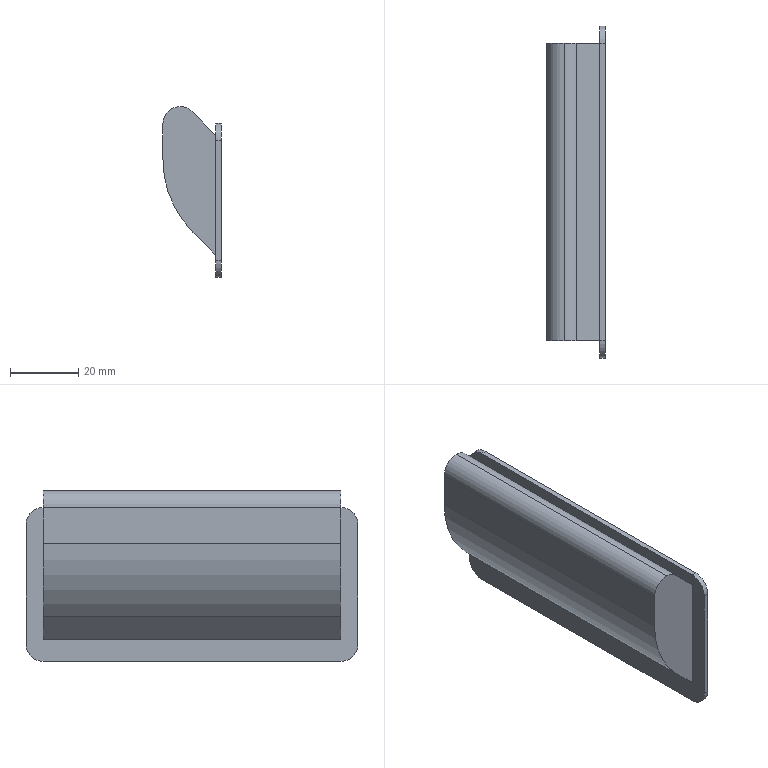Part | SolidWorks | features BaseBody 1 | 1 solid | 23 faces | box 17 x 97 x 49.929 mm | volume 24754 mm3 | plane 14 | cylinder 9 | commonest cylinder face diameters 10 x6 30 x2 60 x1
STEP:
#1=CARTESIAN_POINT('',(5.,-43.5,10.429));
#2=VERTEX_POINT('',#1);
#3=CARTESIAN_POINT('',(0.,-43.5,5.429));
#4=VERTEX_POINT('',#3);
#5=CARTESIAN_POINT('',(5.,-43.5,5.429));
#6=DIRECTION('',(0.,-1.,0.));
#7=DIRECTION('',(0.,0.,1.));
#8=AXIS2_PLACEMENT_3D('',#5,#6,#7);
#9=CIRCLE('',#8,5.);
#10=EDGE_CURVE('',#2,#4,#9,.T.);
#11=ORIENTED_EDGE('',*,*,#10,.F.);
#12=CARTESIAN_POINT('',(5.,43.5,10.429));
#13=VERTEX_POINT('',#12);
#14=CARTESIAN_POINT('',(5.,-43.5,10.429));
#15=DIRECTION('',(0.,1.,0.));
#16=VECTOR('',#15,1000.);
#17=LINE('',#14,#16);
#18=EDGE_CURVE('',#2,#13,#17,.T.);
#19=ORIENTED_EDGE('',*,*,#18,.T.);
#20=CARTESIAN_POINT('',(0.,43.5,5.429));
#21=VERTEX_POINT('',#20);
#22=CARTESIAN_POINT('',(5.,43.5,5.429));
#23=DIRECTION('',(0.,-1.,0.));
#24=DIRECTION('',(0.,0.,1.));
#25=AXIS2_PLACEMENT_3D('',#22,#23,#24);
#26=CIRCLE('',#25,5.);
#27=EDGE_CURVE('',#13,#21,#26,.T.);
#28=ORIENTED_EDGE('',*,*,#27,.T.);
#29=CARTESIAN_POINT('',(0.,-43.5,5.429));
#30=DIRECTION('',(0.,1.,0.));
#31=VECTOR('',#30,1000.);
#32=LINE('',#29,#31);
#33=EDGE_CURVE('',#4,#21,#32,.T.);
#34=ORIENTED_EDGE('',*,*,#33,.F.);
#35=EDGE_LOOP('',(#11,#19,#28,#34));
#36=FACE_OUTER_BOUND('',#35,.T.);
#37=CARTESIAN_POINT('',(5.,-43.5,5.429));
#38=DIRECTION('',(0.,1.,0.));
#39=DIRECTION('',(0.,0.,1.));
#40=AXIS2_PLACEMENT_3D('',#37,#38,#39);
#41=CYLINDRICAL_SURFACE('',#40,5.);
#42=ADVANCED_FACE('',(#36),#41,.T.);
#43=CARTESIAN_POINT('',(8.787,-43.5,-26.287));
#44=VERTEX_POINT('',#43);
#45=CARTESIAN_POINT('',(0.,-43.5,-5.074));
#46=VERTEX_POINT('',#45);
#47=CARTESIAN_POINT('',(30.,-43.5,-5.074));
#48=DIRECTION('',(0.,1.,0.));
#49=DIRECTION('',(0.,0.,1.));
#50=AXIS2_PLACEMENT_3D('',#47,#48,#49);
#51=CIRCLE('',#50,30.);
#52=EDGE_CURVE('',#44,#46,#51,.T.);
#53=ORIENTED_EDGE('',*,*,#52,.T.);
#54=CARTESIAN_POINT('',(0.,43.5,-5.074));
#55=VERTEX_POINT('',#54);
#56=CARTESIAN_POINT('',(0.,-43.5,-5.074));
#57=DIRECTION('',(0.,1.,0.));
#58=VECTOR('',#57,1000.);
#59=LINE('',#56,#58);
#60=EDGE_CURVE('',#46,#55,#59,.T.);
#61=ORIENTED_EDGE('',*,*,#60,.T.);
#62=CARTESIAN_POINT('',(8.787,43.5,-26.287));
#63=VERTEX_POINT('',#62);
#64=CARTESIAN_POINT('',(30.,43.5,-5.074));
#65=DIRECTION('',(0.,-1.,0.));
#66=DIRECTION('',(0.,0.,1.));
#67=AXIS2_PLACEMENT_3D('',#64,#65,#66);
#68=CIRCLE('',#67,30.);
#69=EDGE_CURVE('',#55,#63,#68,.T.);
#70=ORIENTED_EDGE('',*,*,#69,.T.);
#71=CARTESIAN_POINT('',(8.787,-43.5,-26.287));
#72=DIRECTION('',(0.,-1.,0.));
#73=VECTOR('',#72,1000.);
#74=LINE('',#71,#73);
#75=EDGE_CURVE('',#63,#44,#74,.T.);
#76=ORIENTED_EDGE('',*,*,#75,.T.);
#77=EDGE_LOOP('',(#53,#61,#70,#76));
#78=FACE_OUTER_BOUND('',#77,.T.);
#79=CARTESIAN_POINT('',(30.,-43.5,-5.074));
#80=DIRECTION('',(0.,1.,0.));
#81=DIRECTION('',(0.,0.,1.));
#82=AXIS2_PLACEMENT_3D('',#79,#80,#81);
#83=CYLINDRICAL_SURFACE('',#82,30.);
#84=ADVANCED_FACE('',(#78),#83,.T.);
#85=CARTESIAN_POINT('',(0.,43.5,-17.5));
#86=DIRECTION('',(0.,0.,-1.));
#87=VECTOR('',#86,1000.);
#88=LINE('',#85,#87);
#89=EDGE_CURVE('',#21,#55,#88,.T.);
#90=ORIENTED_EDGE('',*,*,#89,.T.);
#91=ORIENTED_EDGE('',*,*,#60,.F.);
#92=CARTESIAN_POINT('',(0.,-43.5,-17.5));
#93=DIRECTION('',(0.,0.,1.));
#94=VECTOR('',#93,1000.);
#95=LINE('',#92,#94);
#96=EDGE_CURVE('',#46,#4,#95,.T.);
#97=ORIENTED_EDGE('',*,*,#96,.T.);
#98=ORIENTED_EDGE('',*,*,#33,.T.);
#99=EDGE_LOOP('',(#90,#91,#97,#98));
#100=FACE_OUTER_BOUND('',#99,.T.);
#101=CARTESIAN_POINT('',(0.,-43.5,-17.5));
#102=DIRECTION('',(-1.,0.,0.));
#103=DIRECTION('',(0.,0.,1.));
#104=AXIS2_PLACEMENT_3D('',#101,#102,#103);
#105=PLANE('',#104);
#106=ADVANCED_FACE('',(#100),#105,.T.);
#107=CARTESIAN_POINT('',(8.536,-43.5,8.964));
#108=VERTEX_POINT('',#107);
#109=CARTESIAN_POINT('',(5.,-43.5,5.429));
#110=DIRECTION('',(0.,-1.,0.));
#111=DIRECTION('',(0.,0.,1.));
#112=AXIS2_PLACEMENT_3D('',#109,#110,#111);
#113=CIRCLE('',#112,5.);
#114=EDGE_CURVE('',#108,#2,#113,.T.);
#115=ORIENTED_EDGE('',*,*,#114,.T.);
#116=ORIENTED_EDGE('',*,*,#10,.T.);
#117=ORIENTED_EDGE('',*,*,#96,.F.);
#118=ORIENTED_EDGE('',*,*,#52,.F.);
#119=CARTESIAN_POINT('',(15.5,-43.5,-33.));
#120=VERTEX_POINT('',#119);
#121=CARTESIAN_POINT('',(8.787,-43.5,-26.287));
#122=DIRECTION('',(0.7071,0.,-0.7071));
#123=VECTOR('',#122,1000.);
#124=LINE('',#121,#123);
#125=EDGE_CURVE('',#44,#120,#124,.T.);
#126=ORIENTED_EDGE('',*,*,#125,.T.);
#127=CARTESIAN_POINT('',(15.5,-43.5,2.));
#128=VERTEX_POINT('',#127);
#129=CARTESIAN_POINT('',(15.5,-43.5,0.5));
#130=DIRECTION('',(0.,0.,1.));
#131=VECTOR('',#130,1000.);
#132=LINE('',#129,#131);
#133=EDGE_CURVE('',#120,#128,#132,.T.);
#134=ORIENTED_EDGE('',*,*,#133,.T.);
#135=CARTESIAN_POINT('',(15.5,-43.5,2.));
#136=DIRECTION('',(-0.7071,0.,0.7071));
#137=VECTOR('',#136,1000.);
#138=LINE('',#135,#137);
#139=EDGE_CURVE('',#128,#108,#138,.T.);
#140=ORIENTED_EDGE('',*,*,#139,.T.);
#141=EDGE_LOOP('',(#115,#116,#117,#118,#126,#134,#140));
#142=FACE_OUTER_BOUND('',#141,.T.);
#143=CARTESIAN_POINT('',(17.,-43.5,0.5));
#144=DIRECTION('',(0.,-1.,0.));
#145=DIRECTION('',(0.,0.,-1.));
#146=AXIS2_PLACEMENT_3D('',#143,#144,#145);
#147=PLANE('',#146);
#148=ADVANCED_FACE('',(#142),#147,.T.);
#149=CARTESIAN_POINT('',(15.5,43.5,-33.));
#150=VERTEX_POINT('',#149);
#151=CARTESIAN_POINT('',(15.5,-43.5,-33.));
#152=DIRECTION('',(0.,-1.,0.));
#153=VECTOR('',#152,1000.);
#154=LINE('',#151,#153);
#155=EDGE_CURVE('',#150,#120,#154,.T.);
#156=ORIENTED_EDGE('',*,*,#155,.T.);
#157=ORIENTED_EDGE('',*,*,#125,.F.);
#158=ORIENTED_EDGE('',*,*,#75,.F.);
#159=CARTESIAN_POINT('',(17.,43.5,-34.5));
#160=DIRECTION('',(0.7071,0.,-0.7071));
#161=VECTOR('',#160,1000.);
#162=LINE('',#159,#161);
#163=EDGE_CURVE('',#63,#150,#162,.T.);
#164=ORIENTED_EDGE('',*,*,#163,.T.);
#165=EDGE_LOOP('',(#156,#157,#158,#164));
#166=FACE_OUTER_BOUND('',#165,.T.);
#167=CARTESIAN_POINT('',(17.,-43.5,-34.5));
#168=DIRECTION('',(-0.7071,0.,-0.7071));
#169=DIRECTION('',(-0.7071,0.,0.7071));
#170=AXIS2_PLACEMENT_3D('',#167,#168,#169);
#171=PLANE('',#170);
#172=ADVANCED_FACE('',(#166),#171,.T.);
#173=ORIENTED_EDGE('',*,*,#163,.F.);
#174=ORIENTED_EDGE('',*,*,#69,.F.);
#175=ORIENTED_EDGE('',*,*,#89,.F.);
#176=ORIENTED_EDGE('',*,*,#27,.F.);
#177=CARTESIAN_POINT('',(8.536,43.5,8.964));
#178=VERTEX_POINT('',#177);
#179=CARTESIAN_POINT('',(5.,43.5,5.429));
#180=DIRECTION('',(0.,-1.,0.));
#181=DIRECTION('',(0.,0.,1.));
#182=AXIS2_PLACEMENT_3D('',#179,#180,#181);
#183=CIRCLE('',#182,5.);
#184=EDGE_CURVE('',#178,#13,#183,.T.);
#185=ORIENTED_EDGE('',*,*,#184,.F.);
#186=CARTESIAN_POINT('',(15.5,43.5,2.));
#187=VERTEX_POINT('',#186);
#188=CARTESIAN_POINT('',(15.5,43.5,2.));
#189=DIRECTION('',(-0.7071,0.,0.7071));
#190=VECTOR('',#189,1000.);
#191=LINE('',#188,#190);
#192=EDGE_CURVE('',#187,#178,#191,.T.);
#193=ORIENTED_EDGE('',*,*,#192,.F.);
#194=CARTESIAN_POINT('',(15.5,43.5,0.5));
#195=DIRECTION('',(0.,0.,1.));
#196=VECTOR('',#195,1000.);
#197=LINE('',#194,#196);
#198=EDGE_CURVE('',#150,#187,#197,.T.);
#199=ORIENTED_EDGE('',*,*,#198,.F.);
#200=EDGE_LOOP('',(#173,#174,#175,#176,#185,#193,#199));
#201=FACE_OUTER_BOUND('',#200,.T.);
#202=CARTESIAN_POINT('',(17.,43.5,0.5));
#203=DIRECTION('',(0.,-1.,0.));
#204=DIRECTION('',(0.,0.,-1.));
#205=AXIS2_PLACEMENT_3D('',#202,#203,#204);
#206=PLANE('',#205);
#207=ADVANCED_FACE('',(#201),#206,.F.);
#208=ORIENTED_EDGE('',*,*,#18,.F.);
#209=ORIENTED_EDGE('',*,*,#114,.F.);
#210=CARTESIAN_POINT('',(8.536,-43.5,8.964));
#211=DIRECTION('',(0.,1.,0.));
#212=VECTOR('',#211,1000.);
#213=LINE('',#210,#212);
#214=EDGE_CURVE('',#108,#178,#213,.T.);
#215=ORIENTED_EDGE('',*,*,#214,.T.);
#216=ORIENTED_EDGE('',*,*,#184,.T.);
#217=EDGE_LOOP('',(#208,#209,#215,#216));
#218=FACE_OUTER_BOUND('',#217,.T.);
#219=CARTESIAN_POINT('',(5.,-43.5,5.429));
#220=DIRECTION('',(0.,1.,0.));
#221=DIRECTION('',(0.,0.,1.));
#222=AXIS2_PLACEMENT_3D('',#219,#220,#221);
#223=CYLINDRICAL_SURFACE('',#222,5.);
#224=ADVANCED_FACE('',(#218),#223,.T.);
#225=CARTESIAN_POINT('',(15.5,-43.5,2.));
#226=DIRECTION('',(0.,1.,0.));
#227=VECTOR('',#226,1000.);
#228=LINE('',#225,#227);
#229=EDGE_CURVE('',#128,#187,#228,.T.);
#230=ORIENTED_EDGE('',*,*,#229,.T.);
#231=ORIENTED_EDGE('',*,*,#192,.T.);
#232=ORIENTED_EDGE('',*,*,#214,.F.);
#233=ORIENTED_EDGE('',*,*,#139,.F.);
#234=EDGE_LOOP('',(#230,#231,#232,#233));
#235=FACE_OUTER_BOUND('',#234,.T.);
#236=CARTESIAN_POINT('',(0.,-43.5,17.5));
#237=DIRECTION('',(0.7071,0.,0.7071));
#238=DIRECTION('',(0.7071,0.,-0.7071));
#239=AXIS2_PLACEMENT_3D('',#236,#237,#238);
#240=PLANE('',#239);
#241=ADVANCED_FACE('',(#235),#240,.T.);
#242=CARTESIAN_POINT('',(15.5,-43.5,5.5));
#243=VERTEX_POINT('',#242);
#244=CARTESIAN_POINT('',(15.5,43.5,5.5));
#245=VERTEX_POINT('',#244);
#246=CARTESIAN_POINT('',(15.5,48.5,5.5));
#247=DIRECTION('',(0.,1.,0.));
#248=VECTOR('',#247,1000.);
#249=LINE('',#246,#248);
#250=EDGE_CURVE('',#243,#245,#249,.T.);
#251=ORIENTED_EDGE('',*,*,#250,.T.);
#252=CARTESIAN_POINT('',(15.5,48.5,0.5));
#253=VERTEX_POINT('',#252);
#254=CARTESIAN_POINT('',(15.5,43.5,0.5));
#255=DIRECTION('',(-1.,0.,0.));
#256=DIRECTION('',(0.,0.,-1.));
#257=AXIS2_PLACEMENT_3D('',#254,#255,#256);
#258=CIRCLE('',#257,5.);
#259=EDGE_CURVE('',#245,#253,#258,.T.);
#260=ORIENTED_EDGE('',*,*,#259,.T.);
#261=CARTESIAN_POINT('',(15.5,48.5,-34.5));
#262=VERTEX_POINT('',#261);
#263=CARTESIAN_POINT('',(15.5,48.5,5.5));
#264=DIRECTION('',(0.,0.,-1.));
#265=VECTOR('',#264,1000.);
#266=LINE('',#263,#265);
#267=EDGE_CURVE('',#253,#262,#266,.T.);
#268=ORIENTED_EDGE('',*,*,#267,.T.);
#269=CARTESIAN_POINT('',(15.5,43.5,-39.5));
#270=VERTEX_POINT('',#269);
#271=CARTESIAN_POINT('',(15.5,43.5,-34.5));
#272=DIRECTION('',(-1.,0.,0.));
#273=DIRECTION('',(0.,0.,-1.));
#274=AXIS2_PLACEMENT_3D('',#271,#272,#273);
#275=CIRCLE('',#274,5.);
#276=EDGE_CURVE('',#262,#270,#275,.T.);
#277=ORIENTED_EDGE('',*,*,#276,.T.);
#278=CARTESIAN_POINT('',(15.5,-43.5,-39.5));
#279=VERTEX_POINT('',#278);
#280=CARTESIAN_POINT('',(15.5,48.5,-39.5));
#281=DIRECTION('',(0.,-1.,0.));
#282=VECTOR('',#281,1000.);
#283=LINE('',#280,#282);
#284=EDGE_CURVE('',#270,#279,#283,.T.);
#285=ORIENTED_EDGE('',*,*,#284,.T.);
#286=CARTESIAN_POINT('',(15.5,-48.5,-34.5));
#287=VERTEX_POINT('',#286);
#288=CARTESIAN_POINT('',(15.5,-43.5,-34.5));
#289=DIRECTION('',(-1.,0.,0.));
#290=DIRECTION('',(0.,0.,-1.));
#291=AXIS2_PLACEMENT_3D('',#288,#289,#290);
#292=CIRCLE('',#291,5.);
#293=EDGE_CURVE('',#279,#287,#292,.T.);
#294=ORIENTED_EDGE('',*,*,#293,.T.);
#295=CARTESIAN_POINT('',(15.5,-48.5,0.5));
#296=VERTEX_POINT('',#295);
#297=CARTESIAN_POINT('',(15.5,-48.5,5.5));
#298=DIRECTION('',(0.,0.,1.));
#299=VECTOR('',#298,1000.);
#300=LINE('',#297,#299);
#301=EDGE_CURVE('',#287,#296,#300,.T.);
#302=ORIENTED_EDGE('',*,*,#301,.T.);
#303=CARTESIAN_POINT('',(15.5,-43.5,0.5));
#304=DIRECTION('',(-1.,0.,0.));
#305=DIRECTION('',(0.,0.,-1.));
#306=AXIS2_PLACEMENT_3D('',#303,#304,#305);
#307=CIRCLE('',#306,5.);
#308=EDGE_CURVE('',#296,#243,#307,.T.);
#309=ORIENTED_EDGE('',*,*,#308,.T.);
#310=EDGE_LOOP('',(#251,#260,#268,#277,#285,#294,#302,#309));
#311=FACE_OUTER_BOUND('',#310,.T.);
#312=ORIENTED_EDGE('',*,*,#229,.F.);
#313=ORIENTED_EDGE('',*,*,#133,.F.);
#314=ORIENTED_EDGE('',*,*,#155,.F.);
#315=ORIENTED_EDGE('',*,*,#198,.T.);
#316=EDGE_LOOP('',(#312,#313,#314,#315));
#317=FACE_BOUND('',#316,.T.);
#318=CARTESIAN_POINT('',(15.5,48.5,5.5));
#319=DIRECTION('',(-1.,0.,0.));
#320=DIRECTION('',(0.,0.,1.));
#321=AXIS2_PLACEMENT_3D('',#318,#319,#320);
#322=PLANE('',#321);
#323=ADVANCED_FACE('',(#311,#317),#322,.T.);
#324=ORIENTED_EDGE('',*,*,#259,.F.);
#325=CARTESIAN_POINT('',(17.,43.5,5.5));
#326=VERTEX_POINT('',#325);
#327=CARTESIAN_POINT('',(15.5,43.5,5.5));
#328=DIRECTION('',(1.,0.,0.));
#329=VECTOR('',#328,1000.);
#330=LINE('',#327,#329);
#331=EDGE_CURVE('',#245,#326,#330,.T.);
#332=ORIENTED_EDGE('',*,*,#331,.T.);
#333=CARTESIAN_POINT('',(17.,48.5,0.5));
#334=VERTEX_POINT('',#333);
#335=CARTESIAN_POINT('',(17.,43.5,0.5));
#336=DIRECTION('',(-1.,0.,0.));
#337=DIRECTION('',(0.,0.,-1.));
#338=AXIS2_PLACEMENT_3D('',#335,#336,#337);
#339=CIRCLE('',#338,5.);
#340=EDGE_CURVE('',#326,#334,#339,.T.);
#341=ORIENTED_EDGE('',*,*,#340,.T.);
#342=CARTESIAN_POINT('',(15.5,48.5,0.5));
#343=DIRECTION('',(-1.,0.,0.));
#344=VECTOR('',#343,1000.);
#345=LINE('',#342,#344);
#346=EDGE_CURVE('',#334,#253,#345,.T.);
#347=ORIENTED_EDGE('',*,*,#346,.T.);
#348=EDGE_LOOP('',(#324,#332,#341,#347));
#349=FACE_OUTER_BOUND('',#348,.T.);
#350=CARTESIAN_POINT('',(15.5,43.5,0.5));
#351=DIRECTION('',(1.,0.,0.));
#352=DIRECTION('',(0.,0.,-1.));
#353=AXIS2_PLACEMENT_3D('',#350,#351,#352);
#354=CYLINDRICAL_SURFACE('',#353,5.);
#355=ADVANCED_FACE('',(#349),#354,.T.);
#356=ORIENTED_EDGE('',*,*,#250,.F.);
#357=CARTESIAN_POINT('',(17.,-43.5,5.5));
#358=VERTEX_POINT('',#357);
#359=CARTESIAN_POINT('',(15.5,-43.5,5.5));
#360=DIRECTION('',(-1.,0.,0.));
#361=VECTOR('',#360,1000.);
#362=LINE('',#359,#361);
#363=EDGE_CURVE('',#358,#243,#362,.T.);
#364=ORIENTED_EDGE('',*,*,#363,.F.);
#365=CARTESIAN_POINT('',(17.,-48.5,5.5));
#366=DIRECTION('',(0.,-1.,0.));
#367=VECTOR('',#366,1000.);
#368=LINE('',#365,#367);
#369=EDGE_CURVE('',#326,#358,#368,.T.);
#370=ORIENTED_EDGE('',*,*,#369,.F.);
#371=ORIENTED_EDGE('',*,*,#331,.F.);
#372=EDGE_LOOP('',(#356,#364,#370,#371));
#373=FACE_OUTER_BOUND('',#372,.T.);
#374=CARTESIAN_POINT('',(15.5,-48.5,5.5));
#375=DIRECTION('',(0.,0.,-1.));
#376=DIRECTION('',(-1.,0.,0.));
#377=AXIS2_PLACEMENT_3D('',#374,#375,#376);
#378=PLANE('',#377);
#379=ADVANCED_FACE('',(#373),#378,.F.);
#380=ORIENTED_EDGE('',*,*,#308,.F.);
#381=CARTESIAN_POINT('',(17.,-48.5,0.5));
#382=VERTEX_POINT('',#381);
#383=CARTESIAN_POINT('',(15.5,-48.5,0.5));
#384=DIRECTION('',(1.,0.,0.));
#385=VECTOR('',#384,1000.);
#386=LINE('',#383,#385);
#387=EDGE_CURVE('',#296,#382,#386,.T.);
#388=ORIENTED_EDGE('',*,*,#387,.T.);
#389=CARTESIAN_POINT('',(17.,-43.5,0.5));
#390=DIRECTION('',(-1.,0.,0.));
#391=DIRECTION('',(0.,0.,-1.));
#392=AXIS2_PLACEMENT_3D('',#389,#390,#391);
#393=CIRCLE('',#392,5.);
#394=EDGE_CURVE('',#382,#358,#393,.T.);
#395=ORIENTED_EDGE('',*,*,#394,.T.);
#396=ORIENTED_EDGE('',*,*,#363,.T.);
#397=EDGE_LOOP('',(#380,#388,#395,#396));
#398=FACE_OUTER_BOUND('',#397,.T.);
#399=CARTESIAN_POINT('',(15.5,-43.5,0.5));
#400=DIRECTION('',(1.,0.,0.));
#401=DIRECTION('',(0.,0.,-1.));
#402=AXIS2_PLACEMENT_3D('',#399,#400,#401);
#403=CYLINDRICAL_SURFACE('',#402,5.);
#404=ADVANCED_FACE('',(#398),#403,.T.);
#405=CARTESIAN_POINT('',(17.,-48.5,-34.5));
#406=VERTEX_POINT('',#405);
#407=CARTESIAN_POINT('',(17.,-48.5,-39.5));
#408=DIRECTION('',(0.,0.,-1.));
#409=VECTOR('',#408,1000.);
#410=LINE('',#407,#409);
#411=EDGE_CURVE('',#382,#406,#410,.T.);
#412=ORIENTED_EDGE('',*,*,#411,.F.);
#413=ORIENTED_EDGE('',*,*,#387,.F.);
#414=ORIENTED_EDGE('',*,*,#301,.F.);
#415=CARTESIAN_POINT('',(15.5,-48.5,-34.5));
#416=DIRECTION('',(-1.,0.,0.));
#417=VECTOR('',#416,1000.);
#418=LINE('',#415,#417);
#419=EDGE_CURVE('',#406,#287,#418,.T.);
#420=ORIENTED_EDGE('',*,*,#419,.F.);
#421=EDGE_LOOP('',(#412,#413,#414,#420));
#422=FACE_OUTER_BOUND('',#421,.T.);
#423=CARTESIAN_POINT('',(15.5,-48.5,-39.5));
#424=DIRECTION('',(0.,1.,0.));
#425=DIRECTION('',(0.,0.,1.));
#426=AXIS2_PLACEMENT_3D('',#423,#424,#425);
#427=PLANE('',#426);
#428=ADVANCED_FACE('',(#422),#427,.F.);
#429=ORIENTED_EDGE('',*,*,#293,.F.);
#430=CARTESIAN_POINT('',(17.,-43.5,-39.5));
#431=VERTEX_POINT('',#430);
#432=CARTESIAN_POINT('',(15.5,-43.5,-39.5));
#433=DIRECTION('',(1.,0.,0.));
#434=VECTOR('',#433,1000.);
#435=LINE('',#432,#434);
#436=EDGE_CURVE('',#279,#431,#435,.T.);
#437=ORIENTED_EDGE('',*,*,#436,.T.);
#438=CARTESIAN_POINT('',(17.,-43.5,-34.5));
#439=DIRECTION('',(-1.,0.,0.));
#440=DIRECTION('',(0.,0.,-1.));
#441=AXIS2_PLACEMENT_3D('',#438,#439,#440);
#442=CIRCLE('',#441,5.);
#443=EDGE_CURVE('',#431,#406,#442,.T.);
#444=ORIENTED_EDGE('',*,*,#443,.T.);
#445=ORIENTED_EDGE('',*,*,#419,.T.);
#446=EDGE_LOOP('',(#429,#437,#444,#445));
#447=FACE_OUTER_BOUND('',#446,.T.);
#448=CARTESIAN_POINT('',(15.5,-43.5,-34.5));
#449=DIRECTION('',(1.,0.,0.));
#450=DIRECTION('',(0.,0.,-1.));
#451=AXIS2_PLACEMENT_3D('',#448,#449,#450);
#452=CYLINDRICAL_SURFACE('',#451,5.);
#453=ADVANCED_FACE('',(#447),#452,.T.);
#454=ORIENTED_EDGE('',*,*,#284,.F.);
#455=CARTESIAN_POINT('',(17.,43.5,-39.5));
#456=VERTEX_POINT('',#455);
#457=CARTESIAN_POINT('',(15.5,43.5,-39.5));
#458=DIRECTION('',(-1.,0.,0.));
#459=VECTOR('',#458,1000.);
#460=LINE('',#457,#459);
#461=EDGE_CURVE('',#456,#270,#460,.T.);
#462=ORIENTED_EDGE('',*,*,#461,.F.);
#463=CARTESIAN_POINT('',(17.,48.5,-39.5));
#464=DIRECTION('',(0.,1.,0.));
#465=VECTOR('',#464,1000.);
#466=LINE('',#463,#465);
#467=EDGE_CURVE('',#431,#456,#466,.T.);
#468=ORIENTED_EDGE('',*,*,#467,.F.);
#469=ORIENTED_EDGE('',*,*,#436,.F.);
#470=EDGE_LOOP('',(#454,#462,#468,#469));
#471=FACE_OUTER_BOUND('',#470,.T.);
#472=CARTESIAN_POINT('',(15.5,48.5,-39.5));
#473=DIRECTION('',(0.,0.,1.));
#474=DIRECTION('',(0.,-1.,0.));
#475=AXIS2_PLACEMENT_3D('',#472,#473,#474);
#476=PLANE('',#475);
#477=ADVANCED_FACE('',(#471),#476,.F.);
#478=ORIENTED_EDGE('',*,*,#276,.F.);
#479=CARTESIAN_POINT('',(17.,48.5,-34.5));
#480=VERTEX_POINT('',#479);
#481=CARTESIAN_POINT('',(15.5,48.5,-34.5));
#482=DIRECTION('',(1.,0.,0.));
#483=VECTOR('',#482,1000.);
#484=LINE('',#481,#483);
#485=EDGE_CURVE('',#262,#480,#484,.T.);
#486=ORIENTED_EDGE('',*,*,#485,.T.);
#487=CARTESIAN_POINT('',(17.,43.5,-34.5));
#488=DIRECTION('',(-1.,0.,0.));
#489=DIRECTION('',(0.,0.,-1.));
#490=AXIS2_PLACEMENT_3D('',#487,#488,#489);
#491=CIRCLE('',#490,5.);
#492=EDGE_CURVE('',#480,#456,#491,.T.);
#493=ORIENTED_EDGE('',*,*,#492,.T.);
#494=ORIENTED_EDGE('',*,*,#461,.T.);
#495=EDGE_LOOP('',(#478,#486,#493,#494));
#496=FACE_OUTER_BOUND('',#495,.T.);
#497=CARTESIAN_POINT('',(15.5,43.5,-34.5));
#498=DIRECTION('',(1.,0.,0.));
#499=DIRECTION('',(0.,0.,-1.));
#500=AXIS2_PLACEMENT_3D('',#497,#498,#499);
#501=CYLINDRICAL_SURFACE('',#500,5.);
#502=ADVANCED_FACE('',(#496),#501,.T.);
#503=ORIENTED_EDGE('',*,*,#267,.F.);
#504=ORIENTED_EDGE('',*,*,#346,.F.);
#505=CARTESIAN_POINT('',(17.,48.5,5.5));
#506=DIRECTION('',(0.,0.,1.));
#507=VECTOR('',#506,1000.);
#508=LINE('',#505,#507);
#509=EDGE_CURVE('',#480,#334,#508,.T.);
#510=ORIENTED_EDGE('',*,*,#509,.F.);
#511=ORIENTED_EDGE('',*,*,#485,.F.);
#512=EDGE_LOOP('',(#503,#504,#510,#511));
#513=FACE_OUTER_BOUND('',#512,.T.);
#514=CARTESIAN_POINT('',(15.5,48.5,5.5));
#515=DIRECTION('',(0.,-1.,0.));
#516=DIRECTION('',(0.,0.,-1.));
#517=AXIS2_PLACEMENT_3D('',#514,#515,#516);
#518=PLANE('',#517);
#519=ADVANCED_FACE('',(#513),#518,.F.);
#520=CARTESIAN_POINT('',(17.,-42.,-2.328));
#521=VERTEX_POINT('',#520);
#522=CARTESIAN_POINT('',(17.,42.,-2.328));
#523=VERTEX_POINT('',#522);
#524=CARTESIAN_POINT('',(17.,-43.5,-2.328));
#525=DIRECTION('',(0.,1.,0.));
#526=VECTOR('',#525,1000.);
#527=LINE('',#524,#526);
#528=EDGE_CURVE('',#521,#523,#527,.T.);
#529=ORIENTED_EDGE('',*,*,#528,.T.);
#530=CARTESIAN_POINT('',(17.,42.,-31.672));
#531=VERTEX_POINT('',#530);
#532=CARTESIAN_POINT('',(17.,42.,0.5));
#533=DIRECTION('',(0.,0.,-1.));
#534=VECTOR('',#533,1000.);
#535=LINE('',#532,#534);
#536=EDGE_CURVE('',#523,#531,#535,.T.);
#537=ORIENTED_EDGE('',*,*,#536,.T.);
#538=CARTESIAN_POINT('',(17.,-42.,-31.672));
#539=VERTEX_POINT('',#538);
#540=CARTESIAN_POINT('',(17.,-43.5,-31.672));
#541=DIRECTION('',(0.,-1.,0.));
#542=VECTOR('',#541,1000.);
#543=LINE('',#540,#542);
#544=EDGE_CURVE('',#531,#539,#543,.T.);
#545=ORIENTED_EDGE('',*,*,#544,.T.);
#546=CARTESIAN_POINT('',(17.,-42.,0.5));
#547=DIRECTION('',(0.,0.,1.));
#548=VECTOR('',#547,1000.);
#549=LINE('',#546,#548);
#550=EDGE_CURVE('',#539,#521,#549,.T.);
#551=ORIENTED_EDGE('',*,*,#550,.T.);
#552=EDGE_LOOP('',(#529,#537,#545,#551));
#553=FACE_BOUND('',#552,.T.);
#554=ORIENTED_EDGE('',*,*,#509,.T.);
#555=ORIENTED_EDGE('',*,*,#340,.F.);
#556=ORIENTED_EDGE('',*,*,#369,.T.);
#557=ORIENTED_EDGE('',*,*,#394,.F.);
#558=ORIENTED_EDGE('',*,*,#411,.T.);
#559=ORIENTED_EDGE('',*,*,#443,.F.);
#560=ORIENTED_EDGE('',*,*,#467,.T.);
#561=ORIENTED_EDGE('',*,*,#492,.F.);
#562=EDGE_LOOP('',(#554,#555,#556,#557,#558,#559,#560,#561));
#563=FACE_OUTER_BOUND('',#562,.T.);
#564=CARTESIAN_POINT('',(17.,-43.5,0.5));
#565=DIRECTION('',(1.,0.,0.));
#566=DIRECTION('',(0.,0.,-1.));
#567=AXIS2_PLACEMENT_3D('',#564,#565,#566);
#568=PLANE('',#567);
#569=ADVANCED_FACE('',(#553,#563),#568,.T.);
#570=ORIENTED_EDGE('',*,*,#536,.F.);
#571=CARTESIAN_POINT('',(2.,42.,-10.458));
#572=VERTEX_POINT('',#571);
#573=CARTESIAN_POINT('',(15.379,42.,-17.241));
#574=DIRECTION('',(0.,1.,0.));
#575=DIRECTION('',(0.,0.,-1.));
#576=AXIS2_PLACEMENT_3D('',#573,#574,#575);
#577=CIRCLE('',#576,15.);
#578=EDGE_CURVE('',#572,#523,#577,.T.);
#579=ORIENTED_EDGE('',*,*,#578,.F.);
#580=CARTESIAN_POINT('',(6.393,42.,-21.065));
#581=VERTEX_POINT('',#580);
#582=CARTESIAN_POINT('',(17.,42.,-10.458));
#583=DIRECTION('',(0.,1.,0.));
#584=DIRECTION('',(0.,0.,-1.));
#585=AXIS2_PLACEMENT_3D('',#582,#583,#584);
#586=CIRCLE('',#585,15.);
#587=EDGE_CURVE('',#581,#572,#586,.T.);
#588=ORIENTED_EDGE('',*,*,#587,.F.);
#589=CARTESIAN_POINT('',(17.,42.,-31.672));
#590=DIRECTION('',(-0.7071,0.,0.7071));
#591=VECTOR('',#590,1000.);
#592=LINE('',#589,#591);
#593=EDGE_CURVE('',#531,#581,#592,.T.);
#594=ORIENTED_EDGE('',*,*,#593,.F.);
#595=EDGE_LOOP('',(#570,#579,#588,#594));
#596=FACE_OUTER_BOUND('',#595,.T.);
#597=CARTESIAN_POINT('',(17.,42.,0.5));
#598=DIRECTION('',(0.,1.,0.));
#599=DIRECTION('',(0.,0.,1.));
#600=AXIS2_PLACEMENT_3D('',#597,#598,#599);
#601=PLANE('',#600);
#602=ADVANCED_FACE('',(#596),#601,.F.);
#603=ORIENTED_EDGE('',*,*,#578,.T.);
#604=ORIENTED_EDGE('',*,*,#528,.F.);
#605=CARTESIAN_POINT('',(2.,-42.,-10.458));
#606=VERTEX_POINT('',#605);
#607=CARTESIAN_POINT('',(15.379,-42.,-17.241));
#608=DIRECTION('',(0.,1.,0.));
#609=DIRECTION('',(0.,0.,-1.));
#610=AXIS2_PLACEMENT_3D('',#607,#608,#609);
#611=CIRCLE('',#610,15.);
#612=EDGE_CURVE('',#606,#521,#611,.T.);
#613=ORIENTED_EDGE('',*,*,#612,.F.);
#614=CARTESIAN_POINT('',(2.,-43.5,-10.458));
#615=DIRECTION('',(0.,-1.,0.));
#616=VECTOR('',#615,1000.);
#617=LINE('',#614,#616);
#618=EDGE_CURVE('',#572,#606,#617,.T.);
#619=ORIENTED_EDGE('',*,*,#618,.F.);
#620=EDGE_LOOP('',(#603,#604,#613,#619));
#621=FACE_OUTER_BOUND('',#620,.T.);
#622=CARTESIAN_POINT('',(15.379,-43.5,-17.241));
#623=DIRECTION('',(0.,-1.,0.));
#624=DIRECTION('',(0.,0.,-1.));
#625=AXIS2_PLACEMENT_3D('',#622,#623,#624);
#626=CYLINDRICAL_SURFACE('',#625,15.);
#627=ADVANCED_FACE('',(#621),#626,.F.);
#628=CARTESIAN_POINT('',(6.393,-42.,-21.065));
#629=VERTEX_POINT('',#628);
#630=CARTESIAN_POINT('',(17.,-42.,-10.458));
#631=DIRECTION('',(0.,1.,0.));
#632=DIRECTION('',(0.,0.,-1.));
#633=AXIS2_PLACEMENT_3D('',#630,#631,#632);
#634=CIRCLE('',#633,15.);
#635=EDGE_CURVE('',#629,#606,#634,.T.);
#636=ORIENTED_EDGE('',*,*,#635,.T.);
#637=ORIENTED_EDGE('',*,*,#612,.T.);
#638=ORIENTED_EDGE('',*,*,#550,.F.);
#639=CARTESIAN_POINT('',(17.,-42.,-31.672));
#640=DIRECTION('',(-0.7071,0.,0.7071));
#641=VECTOR('',#640,1000.);
#642=LINE('',#639,#641);
#643=EDGE_CURVE('',#539,#629,#642,.T.);
#644=ORIENTED_EDGE('',*,*,#643,.T.);
#645=EDGE_LOOP('',(#636,#637,#638,#644));
#646=FACE_OUTER_BOUND('',#645,.T.);
#647=CARTESIAN_POINT('',(17.,-42.,0.5));
#648=DIRECTION('',(0.,1.,0.));
#649=DIRECTION('',(0.,0.,1.));
#650=AXIS2_PLACEMENT_3D('',#647,#648,#649);
#651=PLANE('',#650);
#652=ADVANCED_FACE('',(#646),#651,.T.);
#653=ORIENTED_EDGE('',*,*,#593,.T.);
#654=CARTESIAN_POINT('',(6.393,-43.5,-21.065));
#655=DIRECTION('',(0.,-1.,0.));
#656=VECTOR('',#655,1000.);
#657=LINE('',#654,#656);
#658=EDGE_CURVE('',#581,#629,#657,.T.);
#659=ORIENTED_EDGE('',*,*,#658,.T.);
#660=ORIENTED_EDGE('',*,*,#643,.F.);
#661=ORIENTED_EDGE('',*,*,#544,.F.);
#662=EDGE_LOOP('',(#653,#659,#660,#661));
#663=FACE_OUTER_BOUND('',#662,.T.);
#664=CARTESIAN_POINT('',(2.,-43.5,-16.672));
#665=DIRECTION('',(0.7071,0.,0.7071));
#666=DIRECTION('',(0.7071,0.,-0.7071));
#667=AXIS2_PLACEMENT_3D('',#664,#665,#666);
#668=PLANE('',#667);
#669=ADVANCED_FACE('',(#663),#668,.T.);
#670=ORIENTED_EDGE('',*,*,#587,.T.);
#671=ORIENTED_EDGE('',*,*,#618,.T.);
#672=ORIENTED_EDGE('',*,*,#635,.F.);
#673=ORIENTED_EDGE('',*,*,#658,.F.);
#674=EDGE_LOOP('',(#670,#671,#672,#673));
#675=FACE_OUTER_BOUND('',#674,.T.);
#676=CARTESIAN_POINT('',(17.,-43.5,-10.458));
#677=DIRECTION('',(0.,-1.,0.));
#678=DIRECTION('',(0.,0.,-1.));
#679=AXIS2_PLACEMENT_3D('',#676,#677,#678);
#680=CYLINDRICAL_SURFACE('',#679,15.);
#681=ADVANCED_FACE('',(#675),#680,.F.);
#682=CLOSED_SHELL('',(#42,#84,#106,#148,#172,#207,#224,#241,#323,#355,#379,#404,#428,#453,#477,#502,#519,#569,#602,#627,#652,#669,#681));
#683=MANIFOLD_SOLID_BREP('',#682);
#684=CARTESIAN_POINT('',(0.,0.,0.));
#685=DIRECTION('',(0.,0.,1.));
#686=DIRECTION('',(1.,0.,0.));
#687=AXIS2_PLACEMENT_3D('',#684,#685,#686);
#688=(LENGTH_UNIT()NAMED_UNIT(*)SI_UNIT(.MILLI.,.METRE.));
#689=UNCERTAINTY_MEASURE_WITH_UNIT(LENGTH_MEASURE(0.00001),#688,'','');
#690=(NAMED_UNIT(*)PLANE_ANGLE_UNIT()SI_UNIT($,.RADIAN.));
#691=(NAMED_UNIT(*)SI_UNIT($,.STERADIAN.)SOLID_ANGLE_UNIT());
#692=(GEOMETRIC_REPRESENTATION_CONTEXT(3)GLOBAL_UNCERTAINTY_ASSIGNED_CONTEXT((#689))GLOBAL_UNIT_ASSIGNED_CONTEXT((#688,#690,#691))REPRESENTATION_CONTEXT('',''));
#693=ADVANCED_BREP_SHAPE_REPRESENTATION('',(#683,#687),#692);